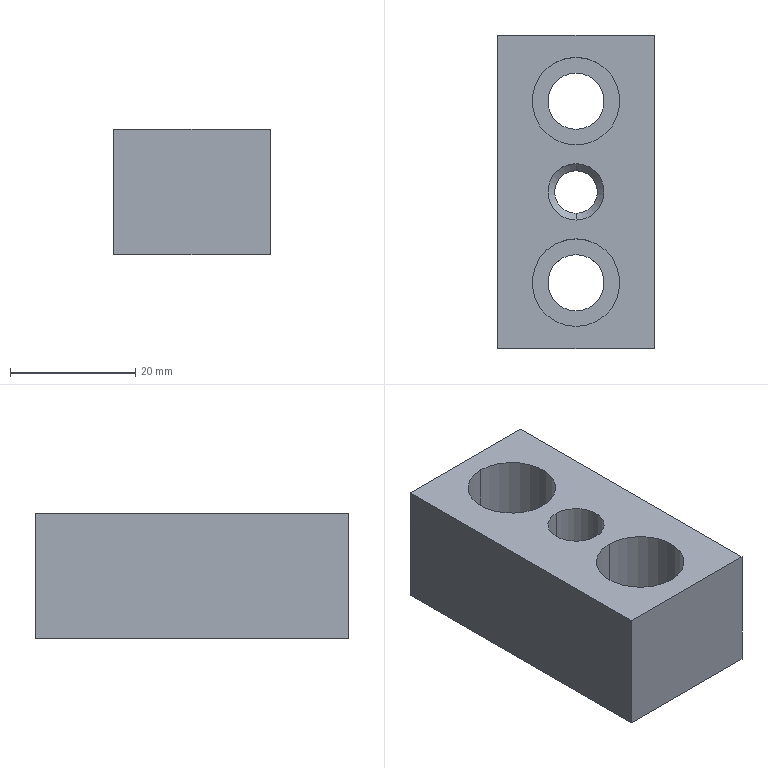Part | STEP file | 1_id1506_x_t | 1 solid | 22 faces | box 25 x 50 x 20 mm | volume 19717 mm3 | cylinder 12 | plane 8 | cone 2 | commonest cylinder face diameters 9 x6 14 x4 6.8 x2